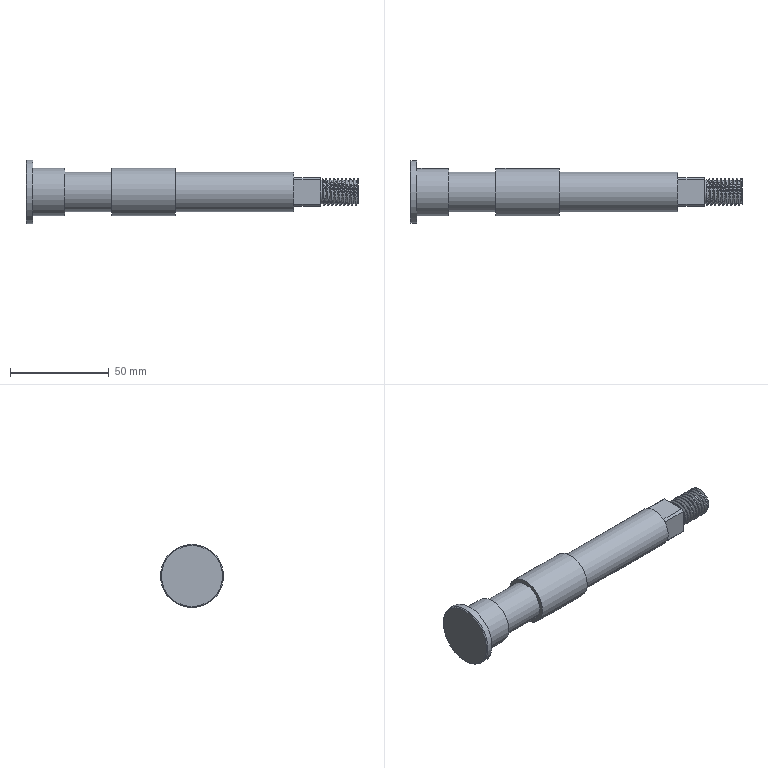Part | NX | features DATUM_CSYS 3, SKETCH 2, CHAMFER 1, EXTRUDE 1, SWP104 1, THREADS 1 | 1 solid | 38 faces | box 168 x 32 x 32 mm | volume 56183 mm3 | cylinder 20 | plane 14 | cone 2 | spline 2 | commonest cylinder face diameters 12 x10 19 x4 20 x2 24 x2 14 x1 32 x1